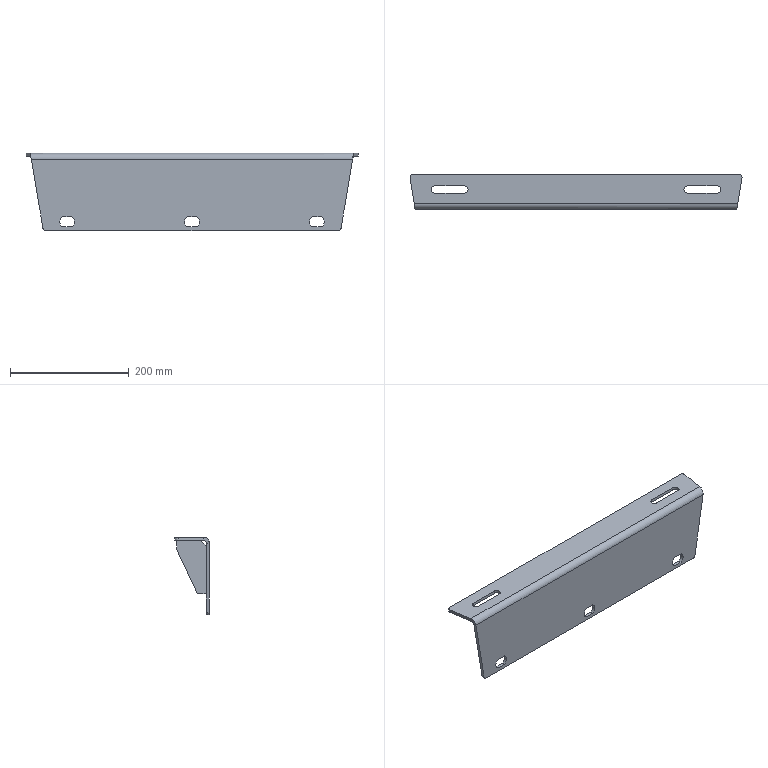Part | SolidWorks | features ICE 2, LPattern 2, Fillet 1, FlatPattern 1, Gusset 1, SM3dBend 1, SMBaseFlange 1, SheetMetal 1 | 3 solids | 54 faces | box 558.195 x 58.219 x 130 mm | volume 495394 mm3 | plane 36 | cylinder 16 | spline 2 | commonest cylinder face diameters 20 x7 10 x5 12 x4